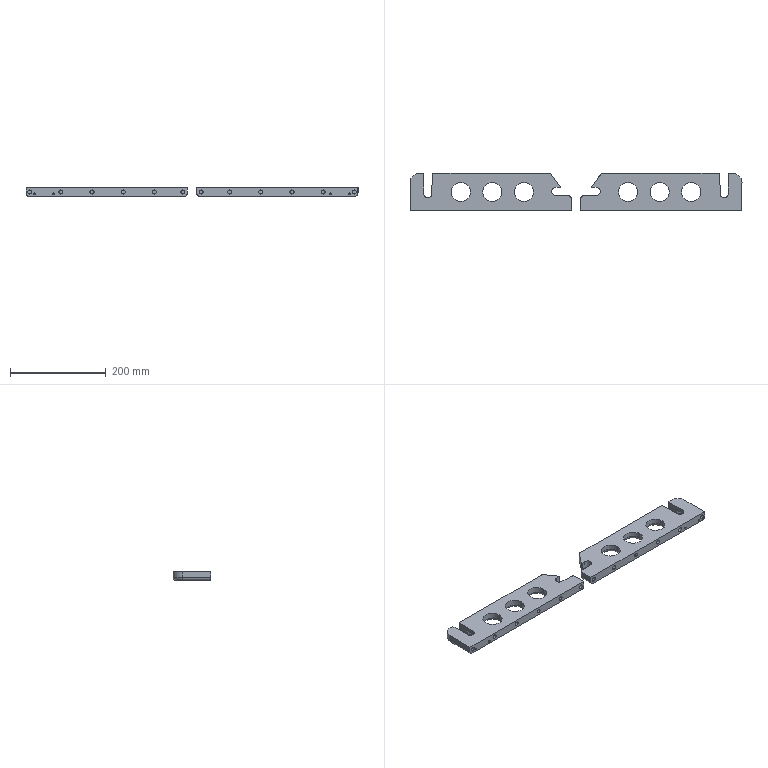Part | 2 solids | 172 faces | box 694.007 x 79 x 18 mm | volume 677028 mm3 | cylinder 94 | plane 46 | spline 16 | torus 16 | commonest cylinder face diameters 8.5 x24 40 x18 4.15 x12 2 x10 4.5 x8 12 x8